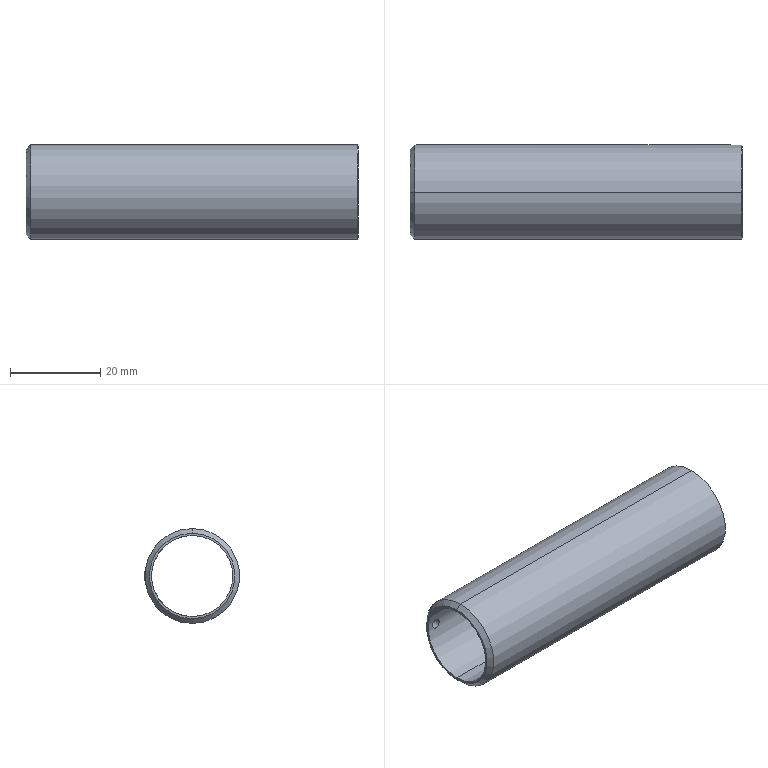Part | STEP file | 2026.6.15-Main Assembly图.sldasm-Part-209 | 1 solid | 23 faces | box 73.5 x 21 x 21 mm | volume 6492 mm3 | cylinder 12 | cone 9 | plane 2 | commonest cylinder face diameters 2.1 x4 18 x2 18.18 x2 18.713 x2 21 x2
STEP:
#1=CARTESIAN_POINT('',(-1554.15,1424.264,3417.176));
#2=VERTEX_POINT('',#1);
#3=CARTESIAN_POINT('',(-1553.688,1424.264,3417.443));
#4=VERTEX_POINT('',#3);
#5=CARTESIAN_POINT('',(-1553.688,1424.264,3417.443));
#6=DIRECTION('',(0.866,0.,0.5));
#7=VECTOR('',#6,1000.);
#8=LINE('',#5,#7);
#9=EDGE_CURVE('',#2,#4,#8,.T.);
#10=ORIENTED_EDGE('',*,*,#9,.F.);
#11=CARTESIAN_POINT('',(-1554.15,1424.264,3398.996));
#12=VERTEX_POINT('',#11);
#13=CARTESIAN_POINT('',(-1554.15,1424.264,3408.086));
#14=DIRECTION('',(-1.,0.,0.));
#15=DIRECTION('',(0.,0.,-1.));
#16=AXIS2_PLACEMENT_3D('',#13,#14,#15);
#17=CIRCLE('',#16,9.09);
#18=EDGE_CURVE('',#2,#12,#17,.T.);
#19=ORIENTED_EDGE('',*,*,#18,.T.);
#20=CARTESIAN_POINT('',(-1553.688,1424.264,3398.73));
#21=VERTEX_POINT('',#20);
#22=CARTESIAN_POINT('',(-1553.688,1424.264,3398.73));
#23=DIRECTION('',(0.866,0.,-0.5));
#24=VECTOR('',#23,1000.);
#25=LINE('',#22,#24);
#26=EDGE_CURVE('',#12,#21,#25,.T.);
#27=ORIENTED_EDGE('',*,*,#26,.T.);
#28=CARTESIAN_POINT('',(-1553.688,1424.264,3408.086));
#29=DIRECTION('',(1.,0.,0.));
#30=DIRECTION('',(0.,0.,-1.));
#31=AXIS2_PLACEMENT_3D('',#28,#29,#30);
#32=CIRCLE('',#31,9.356);
#33=EDGE_CURVE('',#21,#4,#32,.T.);
#34=ORIENTED_EDGE('',*,*,#33,.T.);
#35=EDGE_LOOP('',(#10,#19,#27,#34));
#36=FACE_OUTER_BOUND('',#35,.T.);
#37=CARTESIAN_POINT('',(-1553.688,1424.264,3408.086));
#38=DIRECTION('',(1.,0.,0.));
#39=DIRECTION('',(0.,0.,1.));
#40=AXIS2_PLACEMENT_3D('',#37,#38,#39);
#41=CONICAL_SURFACE('',#40,9.356,0.5236);
#42=ADVANCED_FACE('',(#36),#41,.F.);
#43=CARTESIAN_POINT('',(-1557.924,1424.264,3417.086));
#44=VERTEX_POINT('',#43);
#45=CARTESIAN_POINT('',(-1557.588,1424.264,3417.176));
#46=VERTEX_POINT('',#45);
#47=CARTESIAN_POINT('',(-1557.588,1424.264,3417.176));
#48=DIRECTION('',(0.9659,0.,0.2588));
#49=VECTOR('',#48,1000.);
#50=LINE('',#47,#49);
#51=EDGE_CURVE('',#44,#46,#50,.T.);
#52=ORIENTED_EDGE('',*,*,#51,.F.);
#53=CARTESIAN_POINT('',(-1557.924,1433.225,3408.922));
#54=VERTEX_POINT('',#53);
#55=CARTESIAN_POINT('',(-1557.924,1424.264,3408.086));
#56=DIRECTION('',(-1.,0.,0.));
#57=DIRECTION('',(0.,0.,1.));
#58=AXIS2_PLACEMENT_3D('',#55,#56,#57);
#59=CIRCLE('',#58,9.);
#60=EDGE_CURVE('',#44,#54,#59,.T.);
#61=ORIENTED_EDGE('',*,*,#60,.T.);
#62=CARTESIAN_POINT('',(-1557.588,1433.298,3409.093));
#63=VERTEX_POINT('',#62);
#64=CARTESIAN_POINT('',(-1557.588,1433.298,3409.093));
#65=CARTESIAN_POINT('',(-1557.71,1433.27,3409.056));
#66=CARTESIAN_POINT('',(-1557.822,1433.246,3409.));
#67=CARTESIAN_POINT('',(-1557.924,1433.225,3408.922));
#68=B_SPLINE_CURVE_WITH_KNOTS('',3,(#64,#65,#66,#67),.UNSPECIFIED.,.F.,.F.,(4,4),(0.,0.0003838),.UNSPECIFIED.);
#69=EDGE_CURVE('',#63,#54,#68,.T.);
#70=ORIENTED_EDGE('',*,*,#69,.F.);
#71=CARTESIAN_POINT('',(-1557.588,1424.264,3408.086));
#72=DIRECTION('',(1.,0.,0.));
#73=DIRECTION('',(0.,0.,-1.));
#74=AXIS2_PLACEMENT_3D('',#71,#72,#73);
#75=CIRCLE('',#74,9.09);
#76=EDGE_CURVE('',#63,#46,#75,.T.);
#77=ORIENTED_EDGE('',*,*,#76,.T.);
#78=EDGE_LOOP('',(#52,#61,#70,#77));
#79=FACE_OUTER_BOUND('',#78,.T.);
#80=CARTESIAN_POINT('',(-1557.588,1424.264,3408.086));
#81=DIRECTION('',(1.,0.,0.));
#82=DIRECTION('',(0.,0.,1.));
#83=AXIS2_PLACEMENT_3D('',#80,#81,#82);
#84=CONICAL_SURFACE('',#83,9.09,0.2618);
#85=ADVANCED_FACE('',(#79),#84,.F.);
#86=CARTESIAN_POINT('',(-1546.102,1424.264,3417.443));
#87=VERTEX_POINT('',#86);
#88=CARTESIAN_POINT('',(-1546.102,1424.264,3417.443));
#89=DIRECTION('',(1.,0.,0.));
#90=VECTOR('',#89,1000.);
#91=LINE('',#88,#90);
#92=EDGE_CURVE('',#4,#87,#91,.T.);
#93=ORIENTED_EDGE('',*,*,#92,.F.);
#94=ORIENTED_EDGE('',*,*,#33,.F.);
#95=CARTESIAN_POINT('',(-1546.102,1424.264,3398.73));
#96=VERTEX_POINT('',#95);
#97=CARTESIAN_POINT('',(-1546.102,1424.264,3398.73));
#98=DIRECTION('',(1.,0.,0.));
#99=VECTOR('',#98,1000.);
#100=LINE('',#97,#99);
#101=EDGE_CURVE('',#21,#96,#100,.T.);
#102=ORIENTED_EDGE('',*,*,#101,.T.);
#103=CARTESIAN_POINT('',(-1546.102,1424.264,3408.086));
#104=DIRECTION('',(1.,0.,0.));
#105=DIRECTION('',(0.,0.,-1.));
#106=AXIS2_PLACEMENT_3D('',#103,#104,#105);
#107=CIRCLE('',#106,9.356);
#108=EDGE_CURVE('',#96,#87,#107,.T.);
#109=ORIENTED_EDGE('',*,*,#108,.T.);
#110=EDGE_LOOP('',(#93,#94,#102,#109));
#111=FACE_OUTER_BOUND('',#110,.T.);
#112=CARTESIAN_POINT('',(-1546.102,1424.264,3408.086));
#113=DIRECTION('',(1.,0.,0.));
#114=DIRECTION('',(0.,0.,1.));
#115=AXIS2_PLACEMENT_3D('',#112,#113,#114);
#116=CYLINDRICAL_SURFACE('',#115,9.356);
#117=ADVANCED_FACE('',(#111),#116,.F.);
#118=CARTESIAN_POINT('',(-1545.288,1424.264,3417.176));
#119=DIRECTION('',(1.,0.,0.));
#120=VECTOR('',#119,1000.);
#121=LINE('',#118,#120);
#122=EDGE_CURVE('',#46,#2,#121,.T.);
#123=ORIENTED_EDGE('',*,*,#122,.F.);
#124=ORIENTED_EDGE('',*,*,#76,.F.);
#125=CARTESIAN_POINT('',(-1556.242,1433.354,3408.004));
#126=VERTEX_POINT('',#125);
#127=CARTESIAN_POINT('',(-1557.588,1433.298,3409.093));
#128=CARTESIAN_POINT('',(-1557.506,1433.296,3409.117));
#129=CARTESIAN_POINT('',(-1557.423,1433.294,3409.131));
#130=CARTESIAN_POINT('',(-1557.254,1433.293,3409.139));
#131=CARTESIAN_POINT('',(-1557.168,1433.294,3409.133));
#132=CARTESIAN_POINT('',(-1556.919,1433.299,3409.084));
#133=CARTESIAN_POINT('',(-1556.761,1433.308,3409.01));
#134=CARTESIAN_POINT('',(-1556.496,1433.327,3408.796));
#135=CARTESIAN_POINT('',(-1556.391,1433.338,3408.657));
#136=CARTESIAN_POINT('',(-1556.257,1433.352,3408.347));
#137=CARTESIAN_POINT('',(-1556.228,1433.355,3408.175));
#138=CARTESIAN_POINT('',(-1556.242,1433.354,3408.004));
#139=B_SPLINE_CURVE_WITH_KNOTS('',3,(#127,#128,#129,#130,#131,#132,#133,#134,#135,#136,#137,#138),.UNSPECIFIED.,.F.,.F.,(4,2,2,2,2,4),(0.,0.0002534,0.0005067,0.001013,0.00152,0.002027),.UNSPECIFIED.);
#140=EDGE_CURVE('',#63,#126,#139,.T.);
#141=ORIENTED_EDGE('',*,*,#140,.T.);
#142=CARTESIAN_POINT('',(-1557.588,1433.298,3407.08));
#143=VERTEX_POINT('',#142);
#144=CARTESIAN_POINT('',(-1556.242,1433.354,3408.004));
#145=CARTESIAN_POINT('',(-1556.248,1433.353,3407.925));
#146=CARTESIAN_POINT('',(-1556.262,1433.352,3407.849));
#147=CARTESIAN_POINT('',(-1556.309,1433.346,3407.701));
#148=CARTESIAN_POINT('',(-1556.34,1433.343,3407.628));
#149=CARTESIAN_POINT('',(-1556.457,1433.331,3407.426));
#150=CARTESIAN_POINT('',(-1556.566,1433.321,3407.309));
#151=CARTESIAN_POINT('',(-1556.758,1433.309,3407.177));
#152=CARTESIAN_POINT('',(-1556.827,1433.305,3407.14));
#153=CARTESIAN_POINT('',(-1556.972,1433.299,3407.082));
#154=CARTESIAN_POINT('',(-1557.047,1433.296,3407.061));
#155=CARTESIAN_POINT('',(-1557.28,1433.292,3407.025));
#156=CARTESIAN_POINT('',(-1557.437,1433.293,3407.035));
#157=CARTESIAN_POINT('',(-1557.588,1433.298,3407.08));
#158=B_SPLINE_CURVE_WITH_KNOTS('',3,(#144,#145,#146,#147,#148,#149,#150,#151,#152,#153,#154,#155,#156,#157),.UNSPECIFIED.,.F.,.F.,(4,2,2,2,2,2,4),(0.,0.0002328,0.0004657,0.0009314,0.001164,0.001397,0.001863),.UNSPECIFIED.);
#159=EDGE_CURVE('',#126,#143,#158,.T.);
#160=ORIENTED_EDGE('',*,*,#159,.T.);
#161=CARTESIAN_POINT('',(-1557.588,1424.264,3398.996));
#162=VERTEX_POINT('',#161);
#163=CARTESIAN_POINT('',(-1557.588,1424.264,3408.086));
#164=DIRECTION('',(1.,0.,0.));
#165=DIRECTION('',(0.,0.,-1.));
#166=AXIS2_PLACEMENT_3D('',#163,#164,#165);
#167=CIRCLE('',#166,9.09);
#168=EDGE_CURVE('',#162,#143,#167,.T.);
#169=ORIENTED_EDGE('',*,*,#168,.F.);
#170=CARTESIAN_POINT('',(-1545.288,1424.264,3398.996));
#171=DIRECTION('',(1.,0.,0.));
#172=VECTOR('',#171,1000.);
#173=LINE('',#170,#172);
#174=EDGE_CURVE('',#162,#12,#173,.T.);
#175=ORIENTED_EDGE('',*,*,#174,.T.);
#176=ORIENTED_EDGE('',*,*,#18,.F.);
#177=EDGE_LOOP('',(#123,#124,#141,#160,#169,#175,#176));
#178=FACE_OUTER_BOUND('',#177,.T.);
#179=CARTESIAN_POINT('',(-1545.288,1424.264,3408.086));
#180=DIRECTION('',(1.,0.,0.));
#181=DIRECTION('',(0.,0.,1.));
#182=AXIS2_PLACEMENT_3D('',#179,#180,#181);
#183=CYLINDRICAL_SURFACE('',#182,9.09);
#184=ADVANCED_FACE('',(#178),#183,.F.);
#185=CARTESIAN_POINT('',(-1618.788,1424.264,3399.086));
#186=VERTEX_POINT('',#185);
#187=CARTESIAN_POINT('',(-1557.924,1424.264,3399.086));
#188=VERTEX_POINT('',#187);
#189=CARTESIAN_POINT('',(-1618.788,1424.264,3399.086));
#190=DIRECTION('',(1.,0.,0.));
#191=VECTOR('',#190,1000.);
#192=LINE('',#189,#191);
#193=EDGE_CURVE('',#186,#188,#192,.T.);
#194=ORIENTED_EDGE('',*,*,#193,.T.);
#195=CARTESIAN_POINT('',(-1557.924,1433.225,3407.251));
#196=VERTEX_POINT('',#195);
#197=CARTESIAN_POINT('',(-1557.924,1424.264,3408.086));
#198=DIRECTION('',(-1.,0.,0.));
#199=DIRECTION('',(0.,0.,1.));
#200=AXIS2_PLACEMENT_3D('',#197,#198,#199);
#201=CIRCLE('',#200,9.);
#202=EDGE_CURVE('',#196,#188,#201,.T.);
#203=ORIENTED_EDGE('',*,*,#202,.F.);
#204=CARTESIAN_POINT('',(-1558.335,1433.264,3408.169));
#205=VERTEX_POINT('',#204);
#206=CARTESIAN_POINT('',(-1557.924,1433.225,3407.251));
#207=CARTESIAN_POINT('',(-1557.994,1433.23,3407.304));
#208=CARTESIAN_POINT('',(-1558.056,1433.236,3407.365));
#209=CARTESIAN_POINT('',(-1558.165,1433.246,3407.502));
#210=CARTESIAN_POINT('',(-1558.211,1433.25,3407.578));
#211=CARTESIAN_POINT('',(-1558.282,1433.258,3407.736));
#212=CARTESIAN_POINT('',(-1558.308,1433.261,3407.821));
#213=CARTESIAN_POINT('',(-1558.338,1433.264,3407.994));
#214=CARTESIAN_POINT('',(-1558.342,1433.265,3408.081));
#215=CARTESIAN_POINT('',(-1558.335,1433.264,3408.169));
#216=B_SPLINE_CURVE_WITH_KNOTS('',3,(#206,#207,#208,#209,#210,#211,#212,#213,#214,#215),.UNSPECIFIED.,.F.,.F.,(4,2,2,2,4),(0.,0.0002611,0.0005223,0.0007834,0.001045),.UNSPECIFIED.);
#217=EDGE_CURVE('',#196,#205,#216,.T.);
#218=ORIENTED_EDGE('',*,*,#217,.T.);
#219=CARTESIAN_POINT('',(-1558.335,1433.264,3408.169));
#220=CARTESIAN_POINT('',(-1558.323,1433.263,3408.317));
#221=CARTESIAN_POINT('',(-1558.28,1433.257,3408.46));
#222=CARTESIAN_POINT('',(-1558.14,1433.243,3408.718));
#223=CARTESIAN_POINT('',(-1558.042,1433.234,3408.832));
#224=CARTESIAN_POINT('',(-1557.924,1433.225,3408.922));
#225=B_SPLINE_CURVE_WITH_KNOTS('',3,(#219,#220,#221,#222,#223,#224),.UNSPECIFIED.,.F.,.F.,(4,2,4),(0.,0.0004396,0.0008792),.UNSPECIFIED.);
#226=EDGE_CURVE('',#205,#54,#225,.T.);
#227=ORIENTED_EDGE('',*,*,#226,.T.);
#228=ORIENTED_EDGE('',*,*,#60,.F.);
#229=CARTESIAN_POINT('',(-1618.788,1424.264,3417.086));
#230=VERTEX_POINT('',#229);
#231=CARTESIAN_POINT('',(-1618.788,1424.264,3417.086));
#232=DIRECTION('',(1.,0.,0.));
#233=VECTOR('',#232,1000.);
#234=LINE('',#231,#233);
#235=EDGE_CURVE('',#230,#44,#234,.T.);
#236=ORIENTED_EDGE('',*,*,#235,.F.);
#237=CARTESIAN_POINT('',(-1618.788,1424.264,3408.086));
#238=DIRECTION('',(1.,0.,0.));
#239=DIRECTION('',(0.,0.,1.));
#240=AXIS2_PLACEMENT_3D('',#237,#238,#239);
#241=CIRCLE('',#240,9.);
#242=EDGE_CURVE('',#186,#230,#241,.T.);
#243=ORIENTED_EDGE('',*,*,#242,.F.);
#244=EDGE_LOOP('',(#194,#203,#218,#227,#228,#236,#243));
#245=FACE_OUTER_BOUND('',#244,.T.);
#246=CARTESIAN_POINT('',(-1615.342,1433.264,3408.004));
#247=VERTEX_POINT('',#246);
#248=CARTESIAN_POINT('',(-1617.435,1433.264,3408.169));
#249=VERTEX_POINT('',#248);
#250=CARTESIAN_POINT('',(-1615.342,1433.264,3408.004));
#251=CARTESIAN_POINT('',(-1615.352,1433.263,3407.866));
#252=CARTESIAN_POINT('',(-1615.39,1433.258,3407.732));
#253=CARTESIAN_POINT('',(-1615.515,1433.245,3407.487));
#254=CARTESIAN_POINT('',(-1615.602,1433.237,3407.377));
#255=CARTESIAN_POINT('',(-1615.81,1433.221,3407.199));
#256=CARTESIAN_POINT('',(-1615.933,1433.213,3407.13));
#257=CARTESIAN_POINT('',(-1616.193,1433.204,3407.046));
#258=CARTESIAN_POINT('',(-1616.333,1433.202,3407.029));
#259=CARTESIAN_POINT('',(-1616.607,1433.204,3407.05));
#260=CARTESIAN_POINT('',(-1616.742,1433.209,3407.088));
#261=CARTESIAN_POINT('',(-1616.987,1433.222,3407.213));
#262=CARTESIAN_POINT('',(-1617.096,1433.23,3407.298));
#263=CARTESIAN_POINT('',(-1617.276,1433.246,3407.509));
#264=CARTESIAN_POINT('',(-1617.344,1433.254,3407.63));
#265=CARTESIAN_POINT('',(-1617.429,1433.263,3407.892));
#266=CARTESIAN_POINT('',(-1617.446,1433.265,3408.03));
#267=CARTESIAN_POINT('',(-1617.435,1433.264,3408.169));
#268=B_SPLINE_CURVE_WITH_KNOTS('',3,(#250,#251,#252,#253,#254,#255,#256,#257,#258,#259,#260,#261,#262,#263,#264,#265,#266,#267),.UNSPECIFIED.,.F.,.F.,(4,2,2,2,2,2,2,2,4),(0.,0.0004106,0.0008212,0.001232,0.001642,0.002053,0.002464,0.002874,0.003285),.UNSPECIFIED.);
#269=EDGE_CURVE('',#247,#249,#268,.T.);
#270=ORIENTED_EDGE('',*,*,#269,.T.);
#271=CARTESIAN_POINT('',(-1617.435,1433.264,3408.169));
#272=CARTESIAN_POINT('',(-1617.424,1433.263,3408.307));
#273=CARTESIAN_POINT('',(-1617.386,1433.258,3408.441));
#274=CARTESIAN_POINT('',(-1617.261,1433.245,3408.686));
#275=CARTESIAN_POINT('',(-1617.174,1433.237,3408.796));
#276=CARTESIAN_POINT('',(-1616.966,1433.221,3408.974));
#277=CARTESIAN_POINT('',(-1616.843,1433.213,3409.042));
#278=CARTESIAN_POINT('',(-1616.583,1433.204,3409.127));
#279=CARTESIAN_POINT('',(-1616.443,1433.202,3409.144));
#280=CARTESIAN_POINT('',(-1616.17,1433.204,3409.123));
#281=CARTESIAN_POINT('',(-1616.035,1433.209,3409.085));
#282=CARTESIAN_POINT('',(-1615.79,1433.222,3408.96));
#283=CARTESIAN_POINT('',(-1615.68,1433.23,3408.874));
#284=CARTESIAN_POINT('',(-1615.5,1433.246,3408.664));
#285=CARTESIAN_POINT('',(-1615.433,1433.254,3408.542));
#286=CARTESIAN_POINT('',(-1615.347,1433.263,3408.281));
#287=CARTESIAN_POINT('',(-1615.331,1433.265,3408.142));
#288=CARTESIAN_POINT('',(-1615.342,1433.264,3408.004));
#289=B_SPLINE_CURVE_WITH_KNOTS('',3,(#271,#272,#273,#274,#275,#276,#277,#278,#279,#280,#281,#282,#283,#284,#285,#286,#287,#288),.UNSPECIFIED.,.F.,.F.,(4,2,2,2,2,2,2,2,4),(0.,0.0004106,0.0008212,0.001232,0.001642,0.002053,0.002464,0.002874,0.003285),.UNSPECIFIED.);
#290=EDGE_CURVE('',#249,#247,#289,.T.);
#291=ORIENTED_EDGE('',*,*,#290,.T.);
#292=EDGE_LOOP('',(#270,#291));
#293=FACE_BOUND('',#292,.T.);
#294=CARTESIAN_POINT('',(-1618.788,1424.264,3408.086));
#295=DIRECTION('',(-1.,0.,0.));
#296=DIRECTION('',(0.,0.,-1.));
#297=AXIS2_PLACEMENT_3D('',#294,#295,#296);
#298=CYLINDRICAL_SURFACE('',#297,9.);
#299=ADVANCED_FACE('',(#245,#293),#298,.F.);
#300=CARTESIAN_POINT('',(-1545.288,1424.264,3418.256));
#301=VERTEX_POINT('',#300);
#302=CARTESIAN_POINT('',(-1545.288,1424.264,3418.256));
#303=DIRECTION('',(0.7071,0.,0.7071));
#304=VECTOR('',#303,1000.);
#305=LINE('',#302,#304);
#306=EDGE_CURVE('',#87,#301,#305,.T.);
#307=ORIENTED_EDGE('',*,*,#306,.F.);
#308=ORIENTED_EDGE('',*,*,#108,.F.);
#309=CARTESIAN_POINT('',(-1545.288,1424.264,3397.916));
#310=VERTEX_POINT('',#309);
#311=CARTESIAN_POINT('',(-1545.288,1424.264,3397.916));
#312=DIRECTION('',(0.7071,0.,-0.7071));
#313=VECTOR('',#312,1000.);
#314=LINE('',#311,#313);
#315=EDGE_CURVE('',#96,#310,#314,.T.);
#316=ORIENTED_EDGE('',*,*,#315,.T.);
#317=CARTESIAN_POINT('',(-1545.288,1424.264,3408.086));
#318=DIRECTION('',(1.,0.,0.));
#319=DIRECTION('',(0.,0.,-1.));
#320=AXIS2_PLACEMENT_3D('',#317,#318,#319);
#321=CIRCLE('',#320,10.17);
#322=EDGE_CURVE('',#310,#301,#321,.T.);
#323=ORIENTED_EDGE('',*,*,#322,.T.);
#324=EDGE_LOOP('',(#307,#308,#316,#323));
#325=FACE_OUTER_BOUND('',#324,.T.);
#326=CARTESIAN_POINT('',(-1545.288,1424.264,3408.086));
#327=DIRECTION('',(1.,0.,0.));
#328=DIRECTION('',(0.,0.,1.));
#329=AXIS2_PLACEMENT_3D('',#326,#327,#328);
#330=CONICAL_SURFACE('',#329,10.17,0.7854);
#331=ADVANCED_FACE('',(#325),#330,.F.);
#332=CARTESIAN_POINT('',(-1558.335,1434.764,3408.169));
#333=VERTEX_POINT('',#332);
#334=CARTESIAN_POINT('',(-1558.335,1503.538,3408.169));
#335=DIRECTION('',(0.,1.,0.));
#336=VECTOR('',#335,1000.);
#337=LINE('',#334,#336);
#338=EDGE_CURVE('',#205,#333,#337,.T.);
#339=ORIENTED_EDGE('',*,*,#338,.F.);
#340=ORIENTED_EDGE('',*,*,#217,.F.);
#341=CARTESIAN_POINT('',(-1557.924,1433.225,3407.251));
#342=CARTESIAN_POINT('',(-1557.822,1433.246,3407.173));
#343=CARTESIAN_POINT('',(-1557.71,1433.27,3407.116));
#344=CARTESIAN_POINT('',(-1557.588,1433.298,3407.08));
#345=B_SPLINE_CURVE_WITH_KNOTS('',3,(#341,#342,#343,#344),.UNSPECIFIED.,.F.,.F.,(4,4),(0.,0.0003838),.UNSPECIFIED.);
#346=EDGE_CURVE('',#196,#143,#345,.T.);
#347=ORIENTED_EDGE('',*,*,#346,.T.);
#348=ORIENTED_EDGE('',*,*,#159,.F.);
#349=CARTESIAN_POINT('',(-1556.242,1434.764,3408.004));
#350=VERTEX_POINT('',#349);
#351=CARTESIAN_POINT('',(-1556.242,1503.538,3408.004));
#352=DIRECTION('',(0.,1.,0.));
#353=VECTOR('',#352,1000.);
#354=LINE('',#351,#353);
#355=EDGE_CURVE('',#126,#350,#354,.T.);
#356=ORIENTED_EDGE('',*,*,#355,.T.);
#357=CARTESIAN_POINT('',(-1558.335,1434.764,3408.169));
#358=CARTESIAN_POINT('',(-1558.346,1434.765,3408.03));
#359=CARTESIAN_POINT('',(-1558.329,1434.763,3407.892));
#360=CARTESIAN_POINT('',(-1558.244,1434.755,3407.631));
#361=CARTESIAN_POINT('',(-1558.176,1434.749,3407.508));
#362=CARTESIAN_POINT('',(-1557.998,1434.735,3407.3));
#363=CARTESIAN_POINT('',(-1557.887,1434.728,3407.213));
#364=CARTESIAN_POINT('',(-1557.644,1434.717,3407.089));
#365=CARTESIAN_POINT('',(-1557.508,1434.713,3407.05));
#366=CARTESIAN_POINT('',(-1557.235,1434.711,3407.029));
#367=CARTESIAN_POINT('',(-1557.095,1434.713,3407.045));
#368=CARTESIAN_POINT('',(-1556.834,1434.721,3407.13));
#369=CARTESIAN_POINT('',(-1556.712,1434.727,3407.198));
#370=CARTESIAN_POINT('',(-1556.501,1434.741,3407.377));
#371=CARTESIAN_POINT('',(-1556.416,1434.748,3407.486));
#372=CARTESIAN_POINT('',(-1556.29,1434.759,3407.732));
#373=CARTESIAN_POINT('',(-1556.252,1434.763,3407.866));
#374=CARTESIAN_POINT('',(-1556.242,1434.764,3408.004));
#375=B_SPLINE_CURVE_WITH_KNOTS('',3,(#357,#358,#359,#360,#361,#362,#363,#364,#365,#366,#367,#368,#369,#370,#371,#372,#373,#374),.UNSPECIFIED.,.F.,.F.,(4,2,2,2,2,2,2,2,4),(0.,0.0004105,0.000821,0.001232,0.001642,0.002053,0.002463,0.002874,0.003284),.UNSPECIFIED.);
#376=EDGE_CURVE('',#333,#350,#375,.T.);
#377=ORIENTED_EDGE('',*,*,#376,.F.);
#378=EDGE_LOOP('',(#339,#340,#347,#348,#356,#377));
#379=FACE_OUTER_BOUND('',#378,.T.);
#380=CARTESIAN_POINT('',(-1557.288,1503.538,3408.086));
#381=DIRECTION('',(0.,1.,0.));
#382=DIRECTION('',(-0.9969,0.,0.0785));
#383=AXIS2_PLACEMENT_3D('',#380,#381,#382);
#384=CYLINDRICAL_SURFACE('',#383,1.05);
#385=ADVANCED_FACE('',(#379),#384,.F.);
#386=CARTESIAN_POINT('',(-1617.435,1434.764,3408.169));
#387=VERTEX_POINT('',#386);
#388=CARTESIAN_POINT('',(-1617.435,1503.538,3408.169));
#389=DIRECTION('',(0.,1.,0.));
#390=VECTOR('',#389,1000.);
#391=LINE('',#388,#390);
#392=EDGE_CURVE('',#249,#387,#391,.T.);
#393=ORIENTED_EDGE('',*,*,#392,.F.);
#394=ORIENTED_EDGE('',*,*,#269,.F.);
#395=CARTESIAN_POINT('',(-1615.342,1434.764,3408.004));
#396=VERTEX_POINT('',#395);
#397=CARTESIAN_POINT('',(-1615.342,1503.538,3408.004));
#398=DIRECTION('',(0.,1.,0.));
#399=VECTOR('',#398,1000.);
#400=LINE('',#397,#399);
#401=EDGE_CURVE('',#247,#396,#400,.T.);
#402=ORIENTED_EDGE('',*,*,#401,.T.);
#403=CARTESIAN_POINT('',(-1617.435,1434.764,3408.169));
#404=CARTESIAN_POINT('',(-1617.446,1434.765,3408.03));
#405=CARTESIAN_POINT('',(-1617.429,1434.763,3407.892));
#406=CARTESIAN_POINT('',(-1617.344,1434.755,3407.631));
#407=CARTESIAN_POINT('',(-1617.276,1434.749,3407.508));
#408=CARTESIAN_POINT('',(-1617.098,1434.735,3407.3));
#409=CARTESIAN_POINT('',(-1616.987,1434.728,3407.213));
#410=CARTESIAN_POINT('',(-1616.744,1434.717,3407.089));
#411=CARTESIAN_POINT('',(-1616.608,1434.713,3407.05));
#412=CARTESIAN_POINT('',(-1616.335,1434.711,3407.029));
#413=CARTESIAN_POINT('',(-1616.195,1434.713,3407.045));
#414=CARTESIAN_POINT('',(-1615.934,1434.721,3407.13));
#415=CARTESIAN_POINT('',(-1615.812,1434.727,3407.198));
#416=CARTESIAN_POINT('',(-1615.601,1434.741,3407.377));
#417=CARTESIAN_POINT('',(-1615.516,1434.748,3407.486));
#418=CARTESIAN_POINT('',(-1615.39,1434.759,3407.732));
#419=CARTESIAN_POINT('',(-1615.352,1434.763,3407.866));
#420=CARTESIAN_POINT('',(-1615.342,1434.764,3408.004));
#421=B_SPLINE_CURVE_WITH_KNOTS('',3,(#403,#404,#405,#406,#407,#408,#409,#410,#411,#412,#413,#414,#415,#416,#417,#418,#419,#420),.UNSPECIFIED.,.F.,.F.,(4,2,2,2,2,2,2,2,4),(0.,0.0004105,0.000821,0.001232,0.001642,0.002053,0.002463,0.002874,0.003284),.UNSPECIFIED.);
#422=EDGE_CURVE('',#387,#396,#421,.T.);
#423=ORIENTED_EDGE('',*,*,#422,.F.);
#424=EDGE_LOOP('',(#393,#394,#402,#423));
#425=FACE_OUTER_BOUND('',#424,.T.);
#426=CARTESIAN_POINT('',(-1616.388,1503.538,3408.086));
#427=DIRECTION('',(0.,1.,0.));
#428=DIRECTION('',(-0.9969,0.,0.0785));
#429=AXIS2_PLACEMENT_3D('',#426,#427,#428);
#430=CYLINDRICAL_SURFACE('',#429,1.05);
#431=ADVANCED_FACE('',(#425),#430,.F.);
#432=CARTESIAN_POINT('',(-1618.788,1424.264,3398.636));
#433=VERTEX_POINT('',#432);
#434=CARTESIAN_POINT('',(-1618.788,1424.264,3417.536));
#435=VERTEX_POINT('',#434);
#436=CARTESIAN_POINT('',(-1618.788,1424.264,3408.086));
#437=DIRECTION('',(1.,0.,0.));
#438=DIRECTION('',(0.,0.,-1.));
#439=AXIS2_PLACEMENT_3D('',#436,#437,#438);
#440=CIRCLE('',#439,9.45);
#441=EDGE_CURVE('',#433,#435,#440,.T.);
#442=ORIENTED_EDGE('',*,*,#441,.F.);
#443=CARTESIAN_POINT('',(-1618.788,1424.264,3408.086));
#444=DIRECTION('',(1.,0.,0.));
#445=DIRECTION('',(0.,0.,-1.));
#446=AXIS2_PLACEMENT_3D('',#443,#444,#445);
#447=CIRCLE('',#446,9.45);
#448=EDGE_CURVE('',#435,#433,#447,.T.);
#449=ORIENTED_EDGE('',*,*,#448,.F.);
#450=EDGE_LOOP('',(#442,#449));
#451=FACE_OUTER_BOUND('',#450,.T.);
#452=CARTESIAN_POINT('',(-1618.788,1424.264,3408.086));
#453=DIRECTION('',(1.,0.,0.));
#454=DIRECTION('',(0.,0.,1.));
#455=AXIS2_PLACEMENT_3D('',#452,#453,#454);
#456=CIRCLE('',#455,9.);
#457=EDGE_CURVE('',#230,#186,#456,.T.);
#458=ORIENTED_EDGE('',*,*,#457,.T.);
#459=ORIENTED_EDGE('',*,*,#242,.T.);
#460=EDGE_LOOP('',(#458,#459));
#461=FACE_BOUND('',#460,.T.);
#462=CARTESIAN_POINT('',(-1618.788,1424.264,3408.086));
#463=DIRECTION('',(-1.,0.,0.));
#464=DIRECTION('',(0.,0.,1.));
#465=AXIS2_PLACEMENT_3D('',#462,#463,#464);
#466=PLANE('',#465);
#467=ADVANCED_FACE('',(#451,#461),#466,.T.);
#468=CARTESIAN_POINT('',(-1545.288,1424.264,3418.586));
#469=VERTEX_POINT('',#468);
#470=CARTESIAN_POINT('',(-1545.288,1424.264,3397.586));
#471=VERTEX_POINT('',#470);
#472=CARTESIAN_POINT('',(-1545.288,1424.264,3408.086));
#473=DIRECTION('',(-1.,0.,0.));
#474=DIRECTION('',(0.,0.,1.));
#475=AXIS2_PLACEMENT_3D('',#472,#473,#474);
#476=CIRCLE('',#475,10.5);
#477=EDGE_CURVE('',#469,#471,#476,.T.);
#478=ORIENTED_EDGE('',*,*,#477,.F.);
#479=CARTESIAN_POINT('',(-1545.288,1424.264,3408.086));
#480=DIRECTION('',(-1.,0.,0.));
#481=DIRECTION('',(0.,0.,1.));
#482=AXIS2_PLACEMENT_3D('',#479,#480,#481);
#483=CIRCLE('',#482,10.5);
#484=EDGE_CURVE('',#471,#469,#483,.T.);
#485=ORIENTED_EDGE('',*,*,#484,.F.);
#486=EDGE_LOOP('',(#478,#485));
#487=FACE_OUTER_BOUND('',#486,.T.);
#488=ORIENTED_EDGE('',*,*,#322,.F.);
#489=CARTESIAN_POINT('',(-1545.288,1424.264,3408.086));
#490=DIRECTION('',(1.,0.,0.));
#491=DIRECTION('',(0.,0.,-1.));
#492=AXIS2_PLACEMENT_3D('',#489,#490,#491);
#493=CIRCLE('',#492,10.17);
#494=EDGE_CURVE('',#301,#310,#493,.T.);
#495=ORIENTED_EDGE('',*,*,#494,.F.);
#496=EDGE_LOOP('',(#488,#495));
#497=FACE_BOUND('',#496,.T.);
#498=CARTESIAN_POINT('',(-1545.288,1424.264,3408.086));
#499=DIRECTION('',(-1.,0.,0.));
#500=DIRECTION('',(0.,0.,1.));
#501=AXIS2_PLACEMENT_3D('',#498,#499,#500);
#502=PLANE('',#501);
#503=ADVANCED_FACE('',(#487,#497),#502,.F.);
#504=CARTESIAN_POINT('',(-1617.738,1424.264,3418.586));
#505=VERTEX_POINT('',#504);
#506=CARTESIAN_POINT('',(-1617.738,1424.264,3418.586));
#507=DIRECTION('',(0.7071,0.,0.7071));
#508=VECTOR('',#507,1000.);
#509=LINE('',#506,#508);
#510=EDGE_CURVE('',#435,#505,#509,.T.);
#511=ORIENTED_EDGE('',*,*,#510,.F.);
#512=ORIENTED_EDGE('',*,*,#448,.T.);
#513=CARTESIAN_POINT('',(-1617.738,1424.264,3397.586));
#514=VERTEX_POINT('',#513);
#515=CARTESIAN_POINT('',(-1617.738,1424.264,3397.586));
#516=DIRECTION('',(0.7071,0.,-0.7071));
#517=VECTOR('',#516,1000.);
#518=LINE('',#515,#517);
#519=EDGE_CURVE('',#433,#514,#518,.T.);
#520=ORIENTED_EDGE('',*,*,#519,.T.);
#521=CARTESIAN_POINT('',(-1617.738,1424.264,3408.086));
#522=DIRECTION('',(1.,0.,0.));
#523=DIRECTION('',(0.,0.,1.));
#524=AXIS2_PLACEMENT_3D('',#521,#522,#523);
#525=CIRCLE('',#524,10.5);
#526=EDGE_CURVE('',#505,#514,#525,.T.);
#527=ORIENTED_EDGE('',*,*,#526,.F.);
#528=EDGE_LOOP('',(#511,#512,#520,#527));
#529=FACE_OUTER_BOUND('',#528,.T.);
#530=CARTESIAN_POINT('',(-1617.738,1424.264,3408.086));
#531=DIRECTION('',(1.,0.,0.));
#532=DIRECTION('',(0.,0.,1.));
#533=AXIS2_PLACEMENT_3D('',#530,#531,#532);
#534=CONICAL_SURFACE('',#533,10.5,0.7854);
#535=ADVANCED_FACE('',(#529),#534,.T.);
#536=CARTESIAN_POINT('',(-1618.788,1424.264,3397.586));
#537=DIRECTION('',(1.,0.,0.));
#538=VECTOR('',#537,1000.);
#539=LINE('',#536,#538);
#540=EDGE_CURVE('',#514,#471,#539,.T.);
#541=ORIENTED_EDGE('',*,*,#540,.T.);
#542=ORIENTED_EDGE('',*,*,#484,.T.);
#543=CARTESIAN_POINT('',(-1618.788,1424.264,3418.586));
#544=DIRECTION('',(1.,0.,0.));
#545=VECTOR('',#544,1000.);
#546=LINE('',#543,#545);
#547=EDGE_CURVE('',#505,#469,#546,.T.);
#548=ORIENTED_EDGE('',*,*,#547,.F.);
#549=ORIENTED_EDGE('',*,*,#526,.T.);
#550=EDGE_LOOP('',(#541,#542,#548,#549));
#551=FACE_OUTER_BOUND('',#550,.T.);
#552=CARTESIAN_POINT('',(-1618.788,1424.264,3408.086));
#553=DIRECTION('',(-1.,0.,0.));
#554=DIRECTION('',(0.,0.,-1.));
#555=AXIS2_PLACEMENT_3D('',#552,#553,#554);
#556=CYLINDRICAL_SURFACE('',#555,10.5);
#557=ADVANCED_FACE('',(#551),#556,.T.);
#558=CARTESIAN_POINT('',(-1554.15,1424.264,3408.086));
#559=DIRECTION('',(-1.,0.,0.));
#560=DIRECTION('',(0.,0.,-1.));
#561=AXIS2_PLACEMENT_3D('',#558,#559,#560);
#562=CIRCLE('',#561,9.09);
#563=EDGE_CURVE('',#12,#2,#562,.T.);
#564=ORIENTED_EDGE('',*,*,#563,.T.);
#565=ORIENTED_EDGE('',*,*,#9,.T.);
#566=CARTESIAN_POINT('',(-1553.688,1424.264,3408.086));
#567=DIRECTION('',(1.,0.,0.));
#568=DIRECTION('',(0.,0.,-1.));
#569=AXIS2_PLACEMENT_3D('',#566,#567,#568);
#570=CIRCLE('',#569,9.356);
#571=EDGE_CURVE('',#4,#21,#570,.T.);
#572=ORIENTED_EDGE('',*,*,#571,.T.);
#573=ORIENTED_EDGE('',*,*,#26,.F.);
#574=EDGE_LOOP('',(#564,#565,#572,#573));
#575=FACE_OUTER_BOUND('',#574,.T.);
#576=CARTESIAN_POINT('',(-1553.688,1424.264,3408.086));
#577=DIRECTION('',(1.,0.,0.));
#578=DIRECTION('',(0.,0.,1.));
#579=AXIS2_PLACEMENT_3D('',#576,#577,#578);
#580=CONICAL_SURFACE('',#579,9.356,0.5236);
#581=ADVANCED_FACE('',(#575),#580,.F.);
#582=ORIENTED_EDGE('',*,*,#202,.T.);
#583=CARTESIAN_POINT('',(-1557.588,1424.264,3398.996));
#584=DIRECTION('',(0.9659,0.,-0.2588));
#585=VECTOR('',#584,1000.);
#586=LINE('',#583,#585);
#587=EDGE_CURVE('',#188,#162,#586,.T.);
#588=ORIENTED_EDGE('',*,*,#587,.T.);
#589=ORIENTED_EDGE('',*,*,#168,.T.);
#590=ORIENTED_EDGE('',*,*,#346,.F.);
#591=EDGE_LOOP('',(#582,#588,#589,#590));
#592=FACE_OUTER_BOUND('',#591,.T.);
#593=CARTESIAN_POINT('',(-1557.588,1424.264,3408.086));
#594=DIRECTION('',(1.,0.,0.));
#595=DIRECTION('',(0.,0.,1.));
#596=AXIS2_PLACEMENT_3D('',#593,#594,#595);
#597=CONICAL_SURFACE('',#596,9.09,0.2618);
#598=ADVANCED_FACE('',(#592),#597,.F.);
#599=CARTESIAN_POINT('',(-1557.924,1424.264,3408.086));
#600=DIRECTION('',(-1.,0.,0.));
#601=DIRECTION('',(0.,0.,1.));
#602=AXIS2_PLACEMENT_3D('',#599,#600,#601);
#603=CIRCLE('',#602,9.);
#604=EDGE_CURVE('',#188,#44,#603,.T.);
#605=ORIENTED_EDGE('',*,*,#604,.T.);
#606=ORIENTED_EDGE('',*,*,#51,.T.);
#607=CARTESIAN_POINT('',(-1557.588,1424.264,3408.086));
#608=DIRECTION('',(1.,0.,0.));
#609=DIRECTION('',(0.,0.,-1.));
#610=AXIS2_PLACEMENT_3D('',#607,#608,#609);
#611=CIRCLE('',#610,9.09);
#612=EDGE_CURVE('',#46,#162,#611,.T.);
#613=ORIENTED_EDGE('',*,*,#612,.T.);
#614=ORIENTED_EDGE('',*,*,#587,.F.);
#615=EDGE_LOOP('',(#605,#606,#613,#614));
#616=FACE_OUTER_BOUND('',#615,.T.);
#617=CARTESIAN_POINT('',(-1557.588,1424.264,3408.086));
#618=DIRECTION('',(1.,0.,0.));
#619=DIRECTION('',(0.,0.,1.));
#620=AXIS2_PLACEMENT_3D('',#617,#618,#619);
#621=CONICAL_SURFACE('',#620,9.09,0.2618);
#622=ADVANCED_FACE('',(#616),#621,.F.);
#623=ORIENTED_EDGE('',*,*,#571,.F.);
#624=ORIENTED_EDGE('',*,*,#92,.T.);
#625=CARTESIAN_POINT('',(-1546.102,1424.264,3408.086));
#626=DIRECTION('',(1.,0.,0.));
#627=DIRECTION('',(0.,0.,-1.));
#628=AXIS2_PLACEMENT_3D('',#625,#626,#627);
#629=CIRCLE('',#628,9.356);
#630=EDGE_CURVE('',#87,#96,#629,.T.);
#631=ORIENTED_EDGE('',*,*,#630,.T.);
#632=ORIENTED_EDGE('',*,*,#101,.F.);
#633=EDGE_LOOP('',(#623,#624,#631,#632));
#634=FACE_OUTER_BOUND('',#633,.T.);
#635=CARTESIAN_POINT('',(-1546.102,1424.264,3408.086));
#636=DIRECTION('',(1.,0.,0.));
#637=DIRECTION('',(0.,0.,1.));
#638=AXIS2_PLACEMENT_3D('',#635,#636,#637);
#639=CYLINDRICAL_SURFACE('',#638,9.356);
#640=ADVANCED_FACE('',(#634),#639,.F.);
#641=ORIENTED_EDGE('',*,*,#612,.F.);
#642=ORIENTED_EDGE('',*,*,#122,.T.);
#643=ORIENTED_EDGE('',*,*,#563,.F.);
#644=ORIENTED_EDGE('',*,*,#174,.F.);
#645=EDGE_LOOP('',(#641,#642,#643,#644));
#646=FACE_OUTER_BOUND('',#645,.T.);
#647=CARTESIAN_POINT('',(-1545.288,1424.264,3408.086));
#648=DIRECTION('',(1.,0.,0.));
#649=DIRECTION('',(0.,0.,1.));
#650=AXIS2_PLACEMENT_3D('',#647,#648,#649);
#651=CYLINDRICAL_SURFACE('',#650,9.09);
#652=ADVANCED_FACE('',(#646),#651,.F.);
#653=ORIENTED_EDGE('',*,*,#604,.F.);
#654=ORIENTED_EDGE('',*,*,#193,.F.);
#655=ORIENTED_EDGE('',*,*,#457,.F.);
#656=ORIENTED_EDGE('',*,*,#235,.T.);
#657=EDGE_LOOP('',(#653,#654,#655,#656));
#658=FACE_OUTER_BOUND('',#657,.T.);
#659=CARTESIAN_POINT('',(-1618.788,1424.264,3408.086));
#660=DIRECTION('',(-1.,0.,0.));
#661=DIRECTION('',(0.,0.,-1.));
#662=AXIS2_PLACEMENT_3D('',#659,#660,#661);
#663=CYLINDRICAL_SURFACE('',#662,9.);
#664=ADVANCED_FACE('',(#658),#663,.F.);
#665=ORIENTED_EDGE('',*,*,#630,.F.);
#666=ORIENTED_EDGE('',*,*,#306,.T.);
#667=ORIENTED_EDGE('',*,*,#494,.T.);
#668=ORIENTED_EDGE('',*,*,#315,.F.);
#669=EDGE_LOOP('',(#665,#666,#667,#668));
#670=FACE_OUTER_BOUND('',#669,.T.);
#671=CARTESIAN_POINT('',(-1545.288,1424.264,3408.086));
#672=DIRECTION('',(1.,0.,0.));
#673=DIRECTION('',(0.,0.,1.));
#674=AXIS2_PLACEMENT_3D('',#671,#672,#673);
#675=CONICAL_SURFACE('',#674,10.17,0.7854);
#676=ADVANCED_FACE('',(#670),#675,.F.);
#677=ORIENTED_EDGE('',*,*,#226,.F.);
#678=ORIENTED_EDGE('',*,*,#338,.T.);
#679=CARTESIAN_POINT('',(-1556.242,1434.764,3408.004));
#680=CARTESIAN_POINT('',(-1556.231,1434.765,3408.142));
#681=CARTESIAN_POINT('',(-1556.247,1434.763,3408.28));
#682=CARTESIAN_POINT('',(-1556.332,1434.755,3408.542));
#683=CARTESIAN_POINT('',(-1556.401,1434.749,3408.664));
#684=CARTESIAN_POINT('',(-1556.579,1434.735,3408.872));
#685=CARTESIAN_POINT('',(-1556.689,1434.728,3408.96));
#686=CARTESIAN_POINT('',(-1556.933,1434.717,3409.084));
#687=CARTESIAN_POINT('',(-1557.069,1434.713,3409.122));
#688=CARTESIAN_POINT('',(-1557.342,1434.711,3409.144));
#689=CARTESIAN_POINT('',(-1557.481,1434.713,3409.128));
#690=CARTESIAN_POINT('',(-1557.743,1434.721,3409.043));
#691=CARTESIAN_POINT('',(-1557.864,1434.727,3408.975));
#692=CARTESIAN_POINT('',(-1558.075,1434.741,3408.795));
#693=CARTESIAN_POINT('',(-1558.161,1434.748,3408.686));
#694=CARTESIAN_POINT('',(-1558.286,1434.759,3408.441));
#695=CARTESIAN_POINT('',(-1558.324,1434.763,3408.307));
#696=CARTESIAN_POINT('',(-1558.335,1434.764,3408.169));
#697=B_SPLINE_CURVE_WITH_KNOTS('',3,(#679,#680,#681,#682,#683,#684,#685,#686,#687,#688,#689,#690,#691,#692,#693,#694,#695,#696),.UNSPECIFIED.,.F.,.F.,(4,2,2,2,2,2,2,2,4),(0.,0.0004105,0.000821,0.001232,0.001642,0.002053,0.002463,0.002874,0.003284),.UNSPECIFIED.);
#698=EDGE_CURVE('',#350,#333,#697,.T.);
#699=ORIENTED_EDGE('',*,*,#698,.F.);
#700=ORIENTED_EDGE('',*,*,#355,.F.);
#701=ORIENTED_EDGE('',*,*,#140,.F.);
#702=ORIENTED_EDGE('',*,*,#69,.T.);
#703=EDGE_LOOP('',(#677,#678,#699,#700,#701,#702));
#704=FACE_OUTER_BOUND('',#703,.T.);
#705=CARTESIAN_POINT('',(-1557.288,1503.538,3408.086));
#706=DIRECTION('',(0.,1.,0.));
#707=DIRECTION('',(-0.9969,0.,0.0785));
#708=AXIS2_PLACEMENT_3D('',#705,#706,#707);
#709=CYLINDRICAL_SURFACE('',#708,1.05);
#710=ADVANCED_FACE('',(#704),#709,.F.);
#711=ORIENTED_EDGE('',*,*,#290,.F.);
#712=ORIENTED_EDGE('',*,*,#392,.T.);
#713=CARTESIAN_POINT('',(-1615.342,1434.764,3408.004));
#714=CARTESIAN_POINT('',(-1615.331,1434.765,3408.142));
#715=CARTESIAN_POINT('',(-1615.347,1434.763,3408.28));
#716=CARTESIAN_POINT('',(-1615.432,1434.755,3408.542));
#717=CARTESIAN_POINT('',(-1615.501,1434.749,3408.664));
#718=CARTESIAN_POINT('',(-1615.679,1434.735,3408.872));
#719=CARTESIAN_POINT('',(-1615.789,1434.728,3408.96));
#720=CARTESIAN_POINT('',(-1616.033,1434.717,3409.084));
#721=CARTESIAN_POINT('',(-1616.169,1434.713,3409.122));
#722=CARTESIAN_POINT('',(-1616.442,1434.711,3409.144));
#723=CARTESIAN_POINT('',(-1616.581,1434.713,3409.128));
#724=CARTESIAN_POINT('',(-1616.843,1434.721,3409.043));
#725=CARTESIAN_POINT('',(-1616.964,1434.727,3408.975));
#726=CARTESIAN_POINT('',(-1617.175,1434.741,3408.795));
#727=CARTESIAN_POINT('',(-1617.261,1434.748,3408.686));
#728=CARTESIAN_POINT('',(-1617.386,1434.759,3408.441));
#729=CARTESIAN_POINT('',(-1617.424,1434.763,3408.307));
#730=CARTESIAN_POINT('',(-1617.435,1434.764,3408.169));
#731=B_SPLINE_CURVE_WITH_KNOTS('',3,(#713,#714,#715,#716,#717,#718,#719,#720,#721,#722,#723,#724,#725,#726,#727,#728,#729,#730),.UNSPECIFIED.,.F.,.F.,(4,2,2,2,2,2,2,2,4),(0.,0.0004105,0.000821,0.001232,0.001642,0.002053,0.002463,0.002874,0.003284),.UNSPECIFIED.);
#732=EDGE_CURVE('',#396,#387,#731,.T.);
#733=ORIENTED_EDGE('',*,*,#732,.F.);
#734=ORIENTED_EDGE('',*,*,#401,.F.);
#735=EDGE_LOOP('',(#711,#712,#733,#734));
#736=FACE_OUTER_BOUND('',#735,.T.);
#737=CARTESIAN_POINT('',(-1616.388,1503.538,3408.086));
#738=DIRECTION('',(0.,1.,0.));
#739=DIRECTION('',(-0.9969,0.,0.0785));
#740=AXIS2_PLACEMENT_3D('',#737,#738,#739);
#741=CYLINDRICAL_SURFACE('',#740,1.05);
#742=ADVANCED_FACE('',(#736),#741,.F.);
#743=ORIENTED_EDGE('',*,*,#441,.T.);
#744=ORIENTED_EDGE('',*,*,#510,.T.);
#745=CARTESIAN_POINT('',(-1617.738,1424.264,3408.086));
#746=DIRECTION('',(1.,0.,0.));
#747=DIRECTION('',(0.,0.,1.));
#748=AXIS2_PLACEMENT_3D('',#745,#746,#747);
#749=CIRCLE('',#748,10.5);
#750=EDGE_CURVE('',#514,#505,#749,.T.);
#751=ORIENTED_EDGE('',*,*,#750,.F.);
#752=ORIENTED_EDGE('',*,*,#519,.F.);
#753=EDGE_LOOP('',(#743,#744,#751,#752));
#754=FACE_OUTER_BOUND('',#753,.T.);
#755=CARTESIAN_POINT('',(-1617.738,1424.264,3408.086));
#756=DIRECTION('',(1.,0.,0.));
#757=DIRECTION('',(0.,0.,1.));
#758=AXIS2_PLACEMENT_3D('',#755,#756,#757);
#759=CONICAL_SURFACE('',#758,10.5,0.7854);
#760=ADVANCED_FACE('',(#754),#759,.T.);
#761=ORIENTED_EDGE('',*,*,#477,.T.);
#762=ORIENTED_EDGE('',*,*,#540,.F.);
#763=ORIENTED_EDGE('',*,*,#750,.T.);
#764=ORIENTED_EDGE('',*,*,#547,.T.);
#765=EDGE_LOOP('',(#761,#762,#763,#764));
#766=FACE_OUTER_BOUND('',#765,.T.);
#767=ORIENTED_EDGE('',*,*,#698,.T.);
#768=ORIENTED_EDGE('',*,*,#376,.T.);
#769=EDGE_LOOP('',(#767,#768));
#770=FACE_BOUND('',#769,.T.);
#771=ORIENTED_EDGE('',*,*,#732,.T.);
#772=ORIENTED_EDGE('',*,*,#422,.T.);
#773=EDGE_LOOP('',(#771,#772));
#774=FACE_BOUND('',#773,.T.);
#775=CARTESIAN_POINT('',(-1618.788,1424.264,3408.086));
#776=DIRECTION('',(-1.,0.,0.));
#777=DIRECTION('',(0.,0.,-1.));
#778=AXIS2_PLACEMENT_3D('',#775,#776,#777);
#779=CYLINDRICAL_SURFACE('',#778,10.5);
#780=ADVANCED_FACE('',(#766,#770,#774),#779,.T.);
#781=CLOSED_SHELL('',(#42,#85,#117,#184,#299,#331,#385,#431,#467,#503,#535,#557,#581,#598,#622,#640,#652,#664,#676,#710,#742,#760,#780));
#782=MANIFOLD_SOLID_BREP('',#781);
#783=CARTESIAN_POINT('',(0.,0.,0.));
#784=DIRECTION('',(0.,0.,1.));
#785=DIRECTION('',(1.,0.,0.));
#786=AXIS2_PLACEMENT_3D('',#783,#784,#785);
#787=(LENGTH_UNIT()NAMED_UNIT(*)SI_UNIT(.MILLI.,.METRE.));
#788=UNCERTAINTY_MEASURE_WITH_UNIT(LENGTH_MEASURE(0.00001),#787,'','');
#789=(NAMED_UNIT(*)PLANE_ANGLE_UNIT()SI_UNIT($,.RADIAN.));
#790=(NAMED_UNIT(*)SI_UNIT($,.STERADIAN.)SOLID_ANGLE_UNIT());
#791=(GEOMETRIC_REPRESENTATION_CONTEXT(3)GLOBAL_UNCERTAINTY_ASSIGNED_CONTEXT((#788))GLOBAL_UNIT_ASSIGNED_CONTEXT((#787,#789,#790))REPRESENTATION_CONTEXT('',''));
#792=ADVANCED_BREP_SHAPE_REPRESENTATION('',(#782,#786),#791);